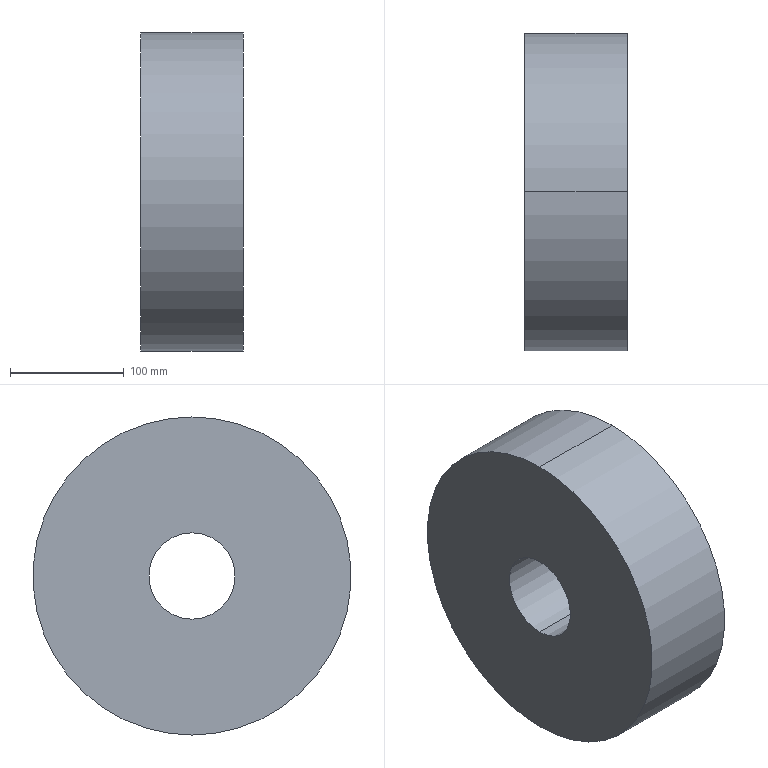Part | SolidWorks | features Revolution 1 | 1 solid | 6 faces | box 90 x 280 x 280 mm | volume 5133488 mm3 | cylinder 4 | plane 2 | commonest cylinder face diameters 76 x2 280 x2
STEP:
#1=CARTESIAN_POINT('',(-45.,0.,-140.));
#2=VERTEX_POINT('',#1);
#3=CARTESIAN_POINT('',(-45.,0.,140.));
#4=VERTEX_POINT('',#3);
#5=CARTESIAN_POINT('',(-45.,0.,0.));
#6=DIRECTION('',(1.,0.,0.));
#7=DIRECTION('',(0.,0.,-1.));
#8=AXIS2_PLACEMENT_3D('',#5,#6,#7);
#9=CIRCLE('',#8,140.);
#10=EDGE_CURVE('',#2,#4,#9,.T.);
#11=ORIENTED_EDGE('',*,*,#10,.T.);
#12=CARTESIAN_POINT('',(45.,0.,140.));
#13=VERTEX_POINT('',#12);
#14=CARTESIAN_POINT('',(71.901,0.,140.));
#15=DIRECTION('',(1.,0.,0.));
#16=VECTOR('',#15,1000.);
#17=LINE('',#14,#16);
#18=EDGE_CURVE('',#4,#13,#17,.T.);
#19=ORIENTED_EDGE('',*,*,#18,.T.);
#20=CARTESIAN_POINT('',(45.,0.,-140.));
#21=VERTEX_POINT('',#20);
#22=CARTESIAN_POINT('',(45.,0.,0.));
#23=DIRECTION('',(1.,0.,0.));
#24=DIRECTION('',(0.,0.,-1.));
#25=AXIS2_PLACEMENT_3D('',#22,#23,#24);
#26=CIRCLE('',#25,140.);
#27=EDGE_CURVE('',#21,#13,#26,.T.);
#28=ORIENTED_EDGE('',*,*,#27,.F.);
#29=CARTESIAN_POINT('',(71.901,0.,-140.));
#30=DIRECTION('',(1.,0.,0.));
#31=VECTOR('',#30,1000.);
#32=LINE('',#29,#31);
#33=EDGE_CURVE('',#2,#21,#32,.T.);
#34=ORIENTED_EDGE('',*,*,#33,.F.);
#35=EDGE_LOOP('',(#11,#19,#28,#34));
#36=FACE_OUTER_BOUND('',#35,.T.);
#37=CARTESIAN_POINT('',(71.901,0.,0.));
#38=DIRECTION('',(1.,0.,0.));
#39=DIRECTION('',(0.,0.,-1.));
#40=AXIS2_PLACEMENT_3D('',#37,#38,#39);
#41=CYLINDRICAL_SURFACE('',#40,140.);
#42=ADVANCED_FACE('',(#36),#41,.T.);
#43=CARTESIAN_POINT('',(-45.,0.,38.));
#44=VERTEX_POINT('',#43);
#45=CARTESIAN_POINT('',(-45.,0.,-38.));
#46=VERTEX_POINT('',#45);
#47=CARTESIAN_POINT('',(-45.,0.,0.));
#48=DIRECTION('',(1.,0.,0.));
#49=DIRECTION('',(0.,0.,-1.));
#50=AXIS2_PLACEMENT_3D('',#47,#48,#49);
#51=CIRCLE('',#50,38.);
#52=EDGE_CURVE('',#44,#46,#51,.T.);
#53=ORIENTED_EDGE('',*,*,#52,.F.);
#54=CARTESIAN_POINT('',(45.,0.,38.));
#55=VERTEX_POINT('',#54);
#56=CARTESIAN_POINT('',(71.901,0.,38.));
#57=DIRECTION('',(1.,0.,0.));
#58=VECTOR('',#57,1000.);
#59=LINE('',#56,#58);
#60=EDGE_CURVE('',#44,#55,#59,.T.);
#61=ORIENTED_EDGE('',*,*,#60,.T.);
#62=CARTESIAN_POINT('',(45.,0.,-38.));
#63=VERTEX_POINT('',#62);
#64=CARTESIAN_POINT('',(45.,0.,0.));
#65=DIRECTION('',(1.,0.,0.));
#66=DIRECTION('',(0.,0.,-1.));
#67=AXIS2_PLACEMENT_3D('',#64,#65,#66);
#68=CIRCLE('',#67,38.);
#69=EDGE_CURVE('',#55,#63,#68,.T.);
#70=ORIENTED_EDGE('',*,*,#69,.T.);
#71=CARTESIAN_POINT('',(71.901,0.,-38.));
#72=DIRECTION('',(1.,0.,0.));
#73=VECTOR('',#72,1000.);
#74=LINE('',#71,#73);
#75=EDGE_CURVE('',#46,#63,#74,.T.);
#76=ORIENTED_EDGE('',*,*,#75,.F.);
#77=EDGE_LOOP('',(#53,#61,#70,#76));
#78=FACE_OUTER_BOUND('',#77,.T.);
#79=CARTESIAN_POINT('',(71.901,0.,0.));
#80=DIRECTION('',(1.,0.,0.));
#81=DIRECTION('',(0.,0.,-1.));
#82=AXIS2_PLACEMENT_3D('',#79,#80,#81);
#83=CYLINDRICAL_SURFACE('',#82,38.);
#84=ADVANCED_FACE('',(#78),#83,.F.);
#85=ORIENTED_EDGE('',*,*,#27,.T.);
#86=CARTESIAN_POINT('',(45.,0.,0.));
#87=DIRECTION('',(1.,0.,0.));
#88=DIRECTION('',(0.,0.,-1.));
#89=AXIS2_PLACEMENT_3D('',#86,#87,#88);
#90=CIRCLE('',#89,140.);
#91=EDGE_CURVE('',#13,#21,#90,.T.);
#92=ORIENTED_EDGE('',*,*,#91,.T.);
#93=EDGE_LOOP('',(#85,#92));
#94=FACE_OUTER_BOUND('',#93,.T.);
#95=CARTESIAN_POINT('',(45.,0.,0.));
#96=DIRECTION('',(1.,0.,0.));
#97=DIRECTION('',(0.,0.,-1.));
#98=AXIS2_PLACEMENT_3D('',#95,#96,#97);
#99=CIRCLE('',#98,38.);
#100=EDGE_CURVE('',#63,#55,#99,.T.);
#101=ORIENTED_EDGE('',*,*,#100,.F.);
#102=ORIENTED_EDGE('',*,*,#69,.F.);
#103=EDGE_LOOP('',(#101,#102));
#104=FACE_BOUND('',#103,.T.);
#105=CARTESIAN_POINT('',(45.,38.,0.));
#106=DIRECTION('',(1.,0.,0.));
#107=DIRECTION('',(0.,0.,-1.));
#108=AXIS2_PLACEMENT_3D('',#105,#106,#107);
#109=PLANE('',#108);
#110=ADVANCED_FACE('',(#94,#104),#109,.T.);
#111=ORIENTED_EDGE('',*,*,#60,.F.);
#112=CARTESIAN_POINT('',(-45.,0.,0.));
#113=DIRECTION('',(1.,0.,0.));
#114=DIRECTION('',(0.,0.,-1.));
#115=AXIS2_PLACEMENT_3D('',#112,#113,#114);
#116=CIRCLE('',#115,38.);
#117=EDGE_CURVE('',#46,#44,#116,.T.);
#118=ORIENTED_EDGE('',*,*,#117,.F.);
#119=ORIENTED_EDGE('',*,*,#75,.T.);
#120=ORIENTED_EDGE('',*,*,#100,.T.);
#121=EDGE_LOOP('',(#111,#118,#119,#120));
#122=FACE_OUTER_BOUND('',#121,.T.);
#123=CARTESIAN_POINT('',(71.901,0.,0.));
#124=DIRECTION('',(1.,0.,0.));
#125=DIRECTION('',(0.,0.,-1.));
#126=AXIS2_PLACEMENT_3D('',#123,#124,#125);
#127=CYLINDRICAL_SURFACE('',#126,38.);
#128=ADVANCED_FACE('',(#122),#127,.F.);
#129=ORIENTED_EDGE('',*,*,#117,.T.);
#130=ORIENTED_EDGE('',*,*,#52,.T.);
#131=EDGE_LOOP('',(#129,#130));
#132=FACE_BOUND('',#131,.T.);
#133=ORIENTED_EDGE('',*,*,#10,.F.);
#134=CARTESIAN_POINT('',(-45.,0.,0.));
#135=DIRECTION('',(1.,0.,0.));
#136=DIRECTION('',(0.,0.,-1.));
#137=AXIS2_PLACEMENT_3D('',#134,#135,#136);
#138=CIRCLE('',#137,140.);
#139=EDGE_CURVE('',#4,#2,#138,.T.);
#140=ORIENTED_EDGE('',*,*,#139,.F.);
#141=EDGE_LOOP('',(#133,#140));
#142=FACE_OUTER_BOUND('',#141,.T.);
#143=CARTESIAN_POINT('',(-45.,38.,0.));
#144=DIRECTION('',(-1.,0.,0.));
#145=DIRECTION('',(0.,0.,1.));
#146=AXIS2_PLACEMENT_3D('',#143,#144,#145);
#147=PLANE('',#146);
#148=ADVANCED_FACE('',(#132,#142),#147,.T.);
#149=ORIENTED_EDGE('',*,*,#18,.F.);
#150=ORIENTED_EDGE('',*,*,#139,.T.);
#151=ORIENTED_EDGE('',*,*,#33,.T.);
#152=ORIENTED_EDGE('',*,*,#91,.F.);
#153=EDGE_LOOP('',(#149,#150,#151,#152));
#154=FACE_OUTER_BOUND('',#153,.T.);
#155=CARTESIAN_POINT('',(71.901,0.,0.));
#156=DIRECTION('',(1.,0.,0.));
#157=DIRECTION('',(0.,0.,-1.));
#158=AXIS2_PLACEMENT_3D('',#155,#156,#157);
#159=CYLINDRICAL_SURFACE('',#158,140.);
#160=ADVANCED_FACE('',(#154),#159,.T.);
#161=CLOSED_SHELL('',(#42,#84,#110,#128,#148,#160));
#162=MANIFOLD_SOLID_BREP('',#161);
#163=CARTESIAN_POINT('',(0.,0.,0.));
#164=DIRECTION('',(0.,0.,1.));
#165=DIRECTION('',(1.,0.,0.));
#166=AXIS2_PLACEMENT_3D('',#163,#164,#165);
#167=(LENGTH_UNIT()NAMED_UNIT(*)SI_UNIT(.MILLI.,.METRE.));
#168=UNCERTAINTY_MEASURE_WITH_UNIT(LENGTH_MEASURE(0.00001),#167,'','');
#169=(NAMED_UNIT(*)PLANE_ANGLE_UNIT()SI_UNIT($,.RADIAN.));
#170=(NAMED_UNIT(*)SI_UNIT($,.STERADIAN.)SOLID_ANGLE_UNIT());
#171=(GEOMETRIC_REPRESENTATION_CONTEXT(3)GLOBAL_UNCERTAINTY_ASSIGNED_CONTEXT((#168))GLOBAL_UNIT_ASSIGNED_CONTEXT((#167,#169,#170))REPRESENTATION_CONTEXT('',''));
#172=ADVANCED_BREP_SHAPE_REPRESENTATION('',(#162,#166),#171);